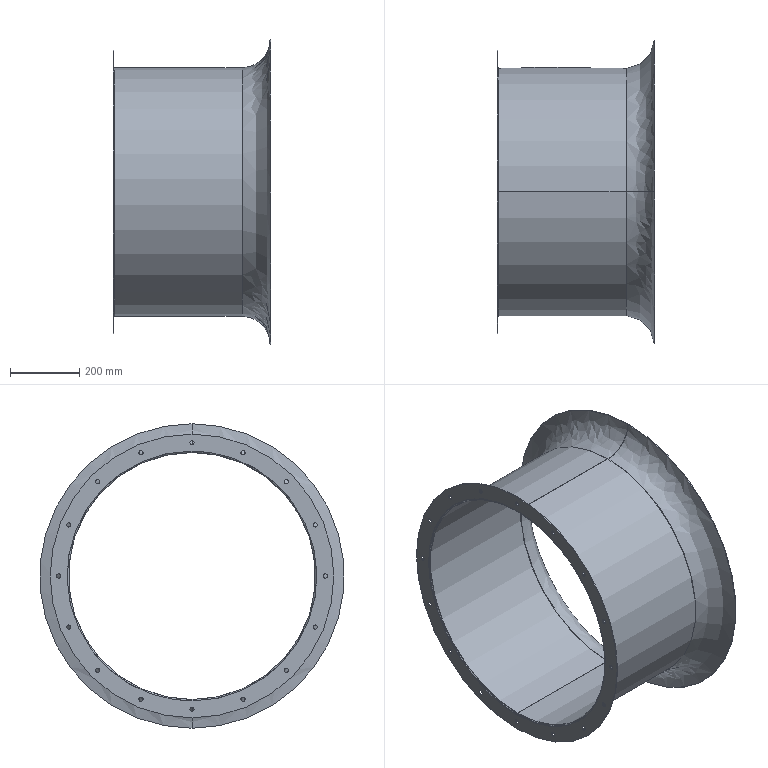Part | STEP file | 750078212 | 1 solid | 58 faces | box 455 x 879 x 879 mm | volume 2524366 mm3 | cylinder 40 | plane 10 | spline 8 | commonest cylinder face diameters 12 x32 713 x2 717 x2 819 x2 879 x2